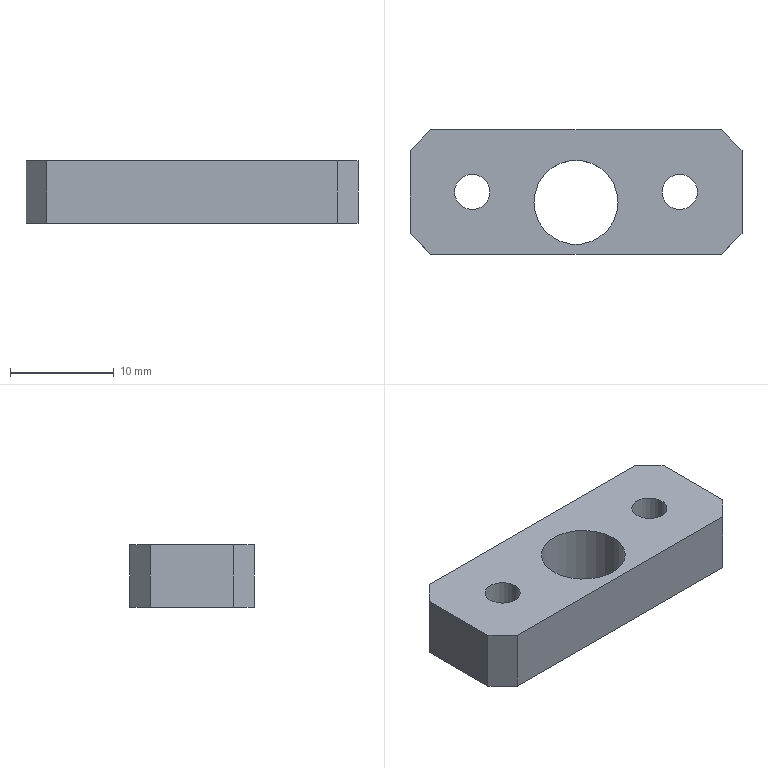Part | STEP file | 11-FG-SZ03211 | 1 solid | 22 faces | box 32 x 12 x 6 mm | volume 1674 mm3 | plane 12 | cylinder 10 | commonest cylinder face diameters 3.4 x4 6.5 x4 8.1 x2
STEP:
#1=CARTESIAN_POINT('',(4.05,-1.,6.));
#2=VERTEX_POINT('',#1);
#3=CARTESIAN_POINT('',(-4.05,-1.,6.));
#4=VERTEX_POINT('',#3);
#5=CARTESIAN_POINT('',(0.,-1.,6.));
#6=DIRECTION('',(0.,0.,-1.));
#7=DIRECTION('',(-1.,0.,0.));
#8=AXIS2_PLACEMENT_3D('',#5,#6,#7);
#9=CIRCLE('',#8,4.05);
#10=EDGE_CURVE('',#2,#4,#9,.T.);
#11=ORIENTED_EDGE('',*,*,#10,.F.);
#12=CARTESIAN_POINT('',(4.05,-1.,0.));
#13=VERTEX_POINT('',#12);
#14=CARTESIAN_POINT('',(4.05,-1.,6.));
#15=DIRECTION('',(0.,0.,-1.));
#16=VECTOR('',#15,1000.);
#17=LINE('',#14,#16);
#18=EDGE_CURVE('',#2,#13,#17,.T.);
#19=ORIENTED_EDGE('',*,*,#18,.T.);
#20=CARTESIAN_POINT('',(-4.05,-1.,0.));
#21=VERTEX_POINT('',#20);
#22=CARTESIAN_POINT('',(0.,-1.,0.));
#23=DIRECTION('',(0.,0.,-1.));
#24=DIRECTION('',(-1.,0.,0.));
#25=AXIS2_PLACEMENT_3D('',#22,#23,#24);
#26=CIRCLE('',#25,4.05);
#27=EDGE_CURVE('',#13,#21,#26,.T.);
#28=ORIENTED_EDGE('',*,*,#27,.T.);
#29=CARTESIAN_POINT('',(-4.05,-1.,6.));
#30=DIRECTION('',(0.,0.,-1.));
#31=VECTOR('',#30,1000.);
#32=LINE('',#29,#31);
#33=EDGE_CURVE('',#4,#21,#32,.T.);
#34=ORIENTED_EDGE('',*,*,#33,.F.);
#35=EDGE_LOOP('',(#11,#19,#28,#34));
#36=FACE_OUTER_BOUND('',#35,.T.);
#37=CARTESIAN_POINT('',(0.,-1.,6.));
#38=DIRECTION('',(0.,0.,-1.));
#39=DIRECTION('',(-1.,0.,0.));
#40=AXIS2_PLACEMENT_3D('',#37,#38,#39);
#41=CYLINDRICAL_SURFACE('',#40,4.05);
#42=ADVANCED_FACE('',(#36),#41,.F.);
#43=CARTESIAN_POINT('',(13.25,0.,3.4));
#44=VERTEX_POINT('',#43);
#45=CARTESIAN_POINT('',(6.75,0.,3.4));
#46=VERTEX_POINT('',#45);
#47=CARTESIAN_POINT('',(10.,0.,3.4));
#48=DIRECTION('',(0.,0.,-1.));
#49=DIRECTION('',(-1.,0.,0.));
#50=AXIS2_PLACEMENT_3D('',#47,#48,#49);
#51=CIRCLE('',#50,3.25);
#52=EDGE_CURVE('',#44,#46,#51,.T.);
#53=ORIENTED_EDGE('',*,*,#52,.F.);
#54=CARTESIAN_POINT('',(13.25,0.,0.));
#55=VERTEX_POINT('',#54);
#56=CARTESIAN_POINT('',(13.25,0.,0.));
#57=DIRECTION('',(0.,0.,-1.));
#58=VECTOR('',#57,1000.);
#59=LINE('',#56,#58);
#60=EDGE_CURVE('',#44,#55,#59,.T.);
#61=ORIENTED_EDGE('',*,*,#60,.T.);
#62=CARTESIAN_POINT('',(6.75,0.,0.));
#63=VERTEX_POINT('',#62);
#64=CARTESIAN_POINT('',(10.,0.,0.));
#65=DIRECTION('',(0.,0.,-1.));
#66=DIRECTION('',(-1.,0.,0.));
#67=AXIS2_PLACEMENT_3D('',#64,#65,#66);
#68=CIRCLE('',#67,3.25);
#69=EDGE_CURVE('',#55,#63,#68,.T.);
#70=ORIENTED_EDGE('',*,*,#69,.T.);
#71=CARTESIAN_POINT('',(6.75,0.,0.));
#72=DIRECTION('',(0.,0.,-1.));
#73=VECTOR('',#72,1000.);
#74=LINE('',#71,#73);
#75=EDGE_CURVE('',#46,#63,#74,.T.);
#76=ORIENTED_EDGE('',*,*,#75,.F.);
#77=EDGE_LOOP('',(#53,#61,#70,#76));
#78=FACE_OUTER_BOUND('',#77,.T.);
#79=CARTESIAN_POINT('',(10.,0.,0.));
#80=DIRECTION('',(0.,0.,-1.));
#81=DIRECTION('',(-1.,0.,0.));
#82=AXIS2_PLACEMENT_3D('',#79,#80,#81);
#83=CYLINDRICAL_SURFACE('',#82,3.25);
#84=ADVANCED_FACE('',(#78),#83,.F.);
#85=CARTESIAN_POINT('',(11.7,0.,6.));
#86=VERTEX_POINT('',#85);
#87=CARTESIAN_POINT('',(8.3,0.,6.));
#88=VERTEX_POINT('',#87);
#89=CARTESIAN_POINT('',(10.,0.,6.));
#90=DIRECTION('',(0.,0.,-1.));
#91=DIRECTION('',(-1.,0.,0.));
#92=AXIS2_PLACEMENT_3D('',#89,#90,#91);
#93=CIRCLE('',#92,1.7);
#94=EDGE_CURVE('',#86,#88,#93,.T.);
#95=ORIENTED_EDGE('',*,*,#94,.F.);
#96=CARTESIAN_POINT('',(11.7,0.,3.4));
#97=VERTEX_POINT('',#96);
#98=CARTESIAN_POINT('',(11.7,0.,0.));
#99=DIRECTION('',(0.,0.,-1.));
#100=VECTOR('',#99,1000.);
#101=LINE('',#98,#100);
#102=EDGE_CURVE('',#86,#97,#101,.T.);
#103=ORIENTED_EDGE('',*,*,#102,.T.);
#104=CARTESIAN_POINT('',(8.3,0.,3.4));
#105=VERTEX_POINT('',#104);
#106=CARTESIAN_POINT('',(10.,0.,3.4));
#107=DIRECTION('',(0.,0.,-1.));
#108=DIRECTION('',(-1.,0.,0.));
#109=AXIS2_PLACEMENT_3D('',#106,#107,#108);
#110=CIRCLE('',#109,1.7);
#111=EDGE_CURVE('',#97,#105,#110,.T.);
#112=ORIENTED_EDGE('',*,*,#111,.T.);
#113=CARTESIAN_POINT('',(8.3,0.,0.));
#114=DIRECTION('',(0.,0.,-1.));
#115=VECTOR('',#114,1000.);
#116=LINE('',#113,#115);
#117=EDGE_CURVE('',#88,#105,#116,.T.);
#118=ORIENTED_EDGE('',*,*,#117,.F.);
#119=EDGE_LOOP('',(#95,#103,#112,#118));
#120=FACE_OUTER_BOUND('',#119,.T.);
#121=CARTESIAN_POINT('',(10.,0.,0.));
#122=DIRECTION('',(0.,0.,-1.));
#123=DIRECTION('',(-1.,0.,0.));
#124=AXIS2_PLACEMENT_3D('',#121,#122,#123);
#125=CYLINDRICAL_SURFACE('',#124,1.7);
#126=ADVANCED_FACE('',(#120),#125,.F.);
#127=CARTESIAN_POINT('',(-6.75,0.,3.4));
#128=VERTEX_POINT('',#127);
#129=CARTESIAN_POINT('',(-13.25,0.,3.4));
#130=VERTEX_POINT('',#129);
#131=CARTESIAN_POINT('',(-10.,0.,3.4));
#132=DIRECTION('',(0.,0.,-1.));
#133=DIRECTION('',(-1.,0.,0.));
#134=AXIS2_PLACEMENT_3D('',#131,#132,#133);
#135=CIRCLE('',#134,3.25);
#136=EDGE_CURVE('',#128,#130,#135,.T.);
#137=ORIENTED_EDGE('',*,*,#136,.F.);
#138=CARTESIAN_POINT('',(-6.75,0.,0.));
#139=VERTEX_POINT('',#138);
#140=CARTESIAN_POINT('',(-6.75,0.,0.));
#141=DIRECTION('',(0.,0.,-1.));
#142=VECTOR('',#141,1000.);
#143=LINE('',#140,#142);
#144=EDGE_CURVE('',#128,#139,#143,.T.);
#145=ORIENTED_EDGE('',*,*,#144,.T.);
#146=CARTESIAN_POINT('',(-13.25,0.,0.));
#147=VERTEX_POINT('',#146);
#148=CARTESIAN_POINT('',(-10.,0.,0.));
#149=DIRECTION('',(0.,0.,-1.));
#150=DIRECTION('',(-1.,0.,0.));
#151=AXIS2_PLACEMENT_3D('',#148,#149,#150);
#152=CIRCLE('',#151,3.25);
#153=EDGE_CURVE('',#139,#147,#152,.T.);
#154=ORIENTED_EDGE('',*,*,#153,.T.);
#155=CARTESIAN_POINT('',(-13.25,0.,0.));
#156=DIRECTION('',(0.,0.,-1.));
#157=VECTOR('',#156,1000.);
#158=LINE('',#155,#157);
#159=EDGE_CURVE('',#130,#147,#158,.T.);
#160=ORIENTED_EDGE('',*,*,#159,.F.);
#161=EDGE_LOOP('',(#137,#145,#154,#160));
#162=FACE_OUTER_BOUND('',#161,.T.);
#163=CARTESIAN_POINT('',(-10.,0.,0.));
#164=DIRECTION('',(0.,0.,-1.));
#165=DIRECTION('',(-1.,0.,0.));
#166=AXIS2_PLACEMENT_3D('',#163,#164,#165);
#167=CYLINDRICAL_SURFACE('',#166,3.25);
#168=ADVANCED_FACE('',(#162),#167,.F.);
#169=CARTESIAN_POINT('',(-8.3,0.,6.));
#170=VERTEX_POINT('',#169);
#171=CARTESIAN_POINT('',(-11.7,0.,6.));
#172=VERTEX_POINT('',#171);
#173=CARTESIAN_POINT('',(-10.,0.,6.));
#174=DIRECTION('',(0.,0.,-1.));
#175=DIRECTION('',(-1.,0.,0.));
#176=AXIS2_PLACEMENT_3D('',#173,#174,#175);
#177=CIRCLE('',#176,1.7);
#178=EDGE_CURVE('',#170,#172,#177,.T.);
#179=ORIENTED_EDGE('',*,*,#178,.F.);
#180=CARTESIAN_POINT('',(-8.3,0.,3.4));
#181=VERTEX_POINT('',#180);
#182=CARTESIAN_POINT('',(-8.3,0.,0.));
#183=DIRECTION('',(0.,0.,-1.));
#184=VECTOR('',#183,1000.);
#185=LINE('',#182,#184);
#186=EDGE_CURVE('',#170,#181,#185,.T.);
#187=ORIENTED_EDGE('',*,*,#186,.T.);
#188=CARTESIAN_POINT('',(-11.7,0.,3.4));
#189=VERTEX_POINT('',#188);
#190=CARTESIAN_POINT('',(-10.,0.,3.4));
#191=DIRECTION('',(0.,0.,-1.));
#192=DIRECTION('',(-1.,0.,0.));
#193=AXIS2_PLACEMENT_3D('',#190,#191,#192);
#194=CIRCLE('',#193,1.7);
#195=EDGE_CURVE('',#181,#189,#194,.T.);
#196=ORIENTED_EDGE('',*,*,#195,.T.);
#197=CARTESIAN_POINT('',(-11.7,0.,0.));
#198=DIRECTION('',(0.,0.,-1.));
#199=VECTOR('',#198,1000.);
#200=LINE('',#197,#199);
#201=EDGE_CURVE('',#172,#189,#200,.T.);
#202=ORIENTED_EDGE('',*,*,#201,.F.);
#203=EDGE_LOOP('',(#179,#187,#196,#202));
#204=FACE_OUTER_BOUND('',#203,.T.);
#205=CARTESIAN_POINT('',(-10.,0.,0.));
#206=DIRECTION('',(0.,0.,-1.));
#207=DIRECTION('',(-1.,0.,0.));
#208=AXIS2_PLACEMENT_3D('',#205,#206,#207);
#209=CYLINDRICAL_SURFACE('',#208,1.7);
#210=ADVANCED_FACE('',(#204),#209,.F.);
#211=CARTESIAN_POINT('',(16.,-4.,6.));
#212=VERTEX_POINT('',#211);
#213=CARTESIAN_POINT('',(16.,4.,6.));
#214=VERTEX_POINT('',#213);
#215=CARTESIAN_POINT('',(16.,6.,6.));
#216=DIRECTION('',(0.,1.,0.));
#217=VECTOR('',#216,1000.);
#218=LINE('',#215,#217);
#219=EDGE_CURVE('',#212,#214,#218,.T.);
#220=ORIENTED_EDGE('',*,*,#219,.F.);
#221=CARTESIAN_POINT('',(16.,-4.,0.));
#222=VERTEX_POINT('',#221);
#223=CARTESIAN_POINT('',(16.,-4.,6.));
#224=DIRECTION('',(0.,0.,-1.));
#225=VECTOR('',#224,1000.);
#226=LINE('',#223,#225);
#227=EDGE_CURVE('',#212,#222,#226,.T.);
#228=ORIENTED_EDGE('',*,*,#227,.T.);
#229=CARTESIAN_POINT('',(16.,4.,0.));
#230=VERTEX_POINT('',#229);
#231=CARTESIAN_POINT('',(16.,6.,0.));
#232=DIRECTION('',(0.,1.,0.));
#233=VECTOR('',#232,1000.);
#234=LINE('',#231,#233);
#235=EDGE_CURVE('',#222,#230,#234,.T.);
#236=ORIENTED_EDGE('',*,*,#235,.T.);
#237=CARTESIAN_POINT('',(16.,4.,6.));
#238=DIRECTION('',(0.,0.,1.));
#239=VECTOR('',#238,1000.);
#240=LINE('',#237,#239);
#241=EDGE_CURVE('',#230,#214,#240,.T.);
#242=ORIENTED_EDGE('',*,*,#241,.T.);
#243=EDGE_LOOP('',(#220,#228,#236,#242));
#244=FACE_OUTER_BOUND('',#243,.T.);
#245=CARTESIAN_POINT('',(16.,6.,6.));
#246=DIRECTION('',(-1.,0.,0.));
#247=DIRECTION('',(0.,0.,1.));
#248=AXIS2_PLACEMENT_3D('',#245,#246,#247);
#249=PLANE('',#248);
#250=ADVANCED_FACE('',(#244),#249,.F.);
#251=CARTESIAN_POINT('',(14.,6.,0.));
#252=VERTEX_POINT('',#251);
#253=CARTESIAN_POINT('',(-14.,6.,0.));
#254=VERTEX_POINT('',#253);
#255=CARTESIAN_POINT('',(-16.,6.,0.));
#256=DIRECTION('',(-1.,0.,0.));
#257=VECTOR('',#256,1000.);
#258=LINE('',#255,#257);
#259=EDGE_CURVE('',#252,#254,#258,.T.);
#260=ORIENTED_EDGE('',*,*,#259,.T.);
#261=CARTESIAN_POINT('',(-14.,6.,6.));
#262=VERTEX_POINT('',#261);
#263=CARTESIAN_POINT('',(-14.,6.,6.));
#264=DIRECTION('',(0.,0.,1.));
#265=VECTOR('',#264,1000.);
#266=LINE('',#263,#265);
#267=EDGE_CURVE('',#254,#262,#266,.T.);
#268=ORIENTED_EDGE('',*,*,#267,.T.);
#269=CARTESIAN_POINT('',(14.,6.,6.));
#270=VERTEX_POINT('',#269);
#271=CARTESIAN_POINT('',(-16.,6.,6.));
#272=DIRECTION('',(-1.,0.,0.));
#273=VECTOR('',#272,1000.);
#274=LINE('',#271,#273);
#275=EDGE_CURVE('',#270,#262,#274,.T.);
#276=ORIENTED_EDGE('',*,*,#275,.F.);
#277=CARTESIAN_POINT('',(14.,6.,6.));
#278=DIRECTION('',(0.,0.,-1.));
#279=VECTOR('',#278,1000.);
#280=LINE('',#277,#279);
#281=EDGE_CURVE('',#270,#252,#280,.T.);
#282=ORIENTED_EDGE('',*,*,#281,.T.);
#283=EDGE_LOOP('',(#260,#268,#276,#282));
#284=FACE_OUTER_BOUND('',#283,.T.);
#285=CARTESIAN_POINT('',(-16.,6.,6.));
#286=DIRECTION('',(0.,-1.,0.));
#287=DIRECTION('',(0.,0.,-1.));
#288=AXIS2_PLACEMENT_3D('',#285,#286,#287);
#289=PLANE('',#288);
#290=ADVANCED_FACE('',(#284),#289,.F.);
#291=CARTESIAN_POINT('',(-16.,4.,0.));
#292=VERTEX_POINT('',#291);
#293=CARTESIAN_POINT('',(-16.,-4.,0.));
#294=VERTEX_POINT('',#293);
#295=CARTESIAN_POINT('',(-16.,6.,0.));
#296=DIRECTION('',(0.,-1.,0.));
#297=VECTOR('',#296,1000.);
#298=LINE('',#295,#297);
#299=EDGE_CURVE('',#292,#294,#298,.T.);
#300=ORIENTED_EDGE('',*,*,#299,.T.);
#301=CARTESIAN_POINT('',(-16.,-4.,6.));
#302=VERTEX_POINT('',#301);
#303=CARTESIAN_POINT('',(-16.,-4.,6.));
#304=DIRECTION('',(0.,0.,1.));
#305=VECTOR('',#304,1000.);
#306=LINE('',#303,#305);
#307=EDGE_CURVE('',#294,#302,#306,.T.);
#308=ORIENTED_EDGE('',*,*,#307,.T.);
#309=CARTESIAN_POINT('',(-16.,4.,6.));
#310=VERTEX_POINT('',#309);
#311=CARTESIAN_POINT('',(-16.,6.,6.));
#312=DIRECTION('',(0.,-1.,0.));
#313=VECTOR('',#312,1000.);
#314=LINE('',#311,#313);
#315=EDGE_CURVE('',#310,#302,#314,.T.);
#316=ORIENTED_EDGE('',*,*,#315,.F.);
#317=CARTESIAN_POINT('',(-16.,4.,6.));
#318=DIRECTION('',(0.,0.,-1.));
#319=VECTOR('',#318,1000.);
#320=LINE('',#317,#319);
#321=EDGE_CURVE('',#310,#292,#320,.T.);
#322=ORIENTED_EDGE('',*,*,#321,.T.);
#323=EDGE_LOOP('',(#300,#308,#316,#322));
#324=FACE_OUTER_BOUND('',#323,.T.);
#325=CARTESIAN_POINT('',(-16.,6.,6.));
#326=DIRECTION('',(1.,0.,0.));
#327=DIRECTION('',(0.,1.,0.));
#328=AXIS2_PLACEMENT_3D('',#325,#326,#327);
#329=PLANE('',#328);
#330=ADVANCED_FACE('',(#324),#329,.F.);
#331=CARTESIAN_POINT('',(-14.,-6.,6.));
#332=VERTEX_POINT('',#331);
#333=CARTESIAN_POINT('',(14.,-6.,6.));
#334=VERTEX_POINT('',#333);
#335=CARTESIAN_POINT('',(-16.,-6.,6.));
#336=DIRECTION('',(1.,0.,0.));
#337=VECTOR('',#336,1000.);
#338=LINE('',#335,#337);
#339=EDGE_CURVE('',#332,#334,#338,.T.);
#340=ORIENTED_EDGE('',*,*,#339,.F.);
#341=CARTESIAN_POINT('',(-14.,-6.,0.));
#342=VERTEX_POINT('',#341);
#343=CARTESIAN_POINT('',(-14.,-6.,6.));
#344=DIRECTION('',(0.,0.,-1.));
#345=VECTOR('',#344,1000.);
#346=LINE('',#343,#345);
#347=EDGE_CURVE('',#332,#342,#346,.T.);
#348=ORIENTED_EDGE('',*,*,#347,.T.);
#349=CARTESIAN_POINT('',(14.,-6.,0.));
#350=VERTEX_POINT('',#349);
#351=CARTESIAN_POINT('',(-16.,-6.,0.));
#352=DIRECTION('',(1.,0.,0.));
#353=VECTOR('',#352,1000.);
#354=LINE('',#351,#353);
#355=EDGE_CURVE('',#342,#350,#354,.T.);
#356=ORIENTED_EDGE('',*,*,#355,.T.);
#357=CARTESIAN_POINT('',(14.,-6.,6.));
#358=DIRECTION('',(0.,0.,1.));
#359=VECTOR('',#358,1000.);
#360=LINE('',#357,#359);
#361=EDGE_CURVE('',#350,#334,#360,.T.);
#362=ORIENTED_EDGE('',*,*,#361,.T.);
#363=EDGE_LOOP('',(#340,#348,#356,#362));
#364=FACE_OUTER_BOUND('',#363,.T.);
#365=CARTESIAN_POINT('',(-16.,-6.,6.));
#366=DIRECTION('',(0.,1.,0.));
#367=DIRECTION('',(0.,0.,1.));
#368=AXIS2_PLACEMENT_3D('',#365,#366,#367);
#369=PLANE('',#368);
#370=ADVANCED_FACE('',(#364),#369,.F.);
#371=CARTESIAN_POINT('',(0.,-1.,6.));
#372=DIRECTION('',(0.,0.,-1.));
#373=DIRECTION('',(-1.,0.,0.));
#374=AXIS2_PLACEMENT_3D('',#371,#372,#373);
#375=CIRCLE('',#374,4.05);
#376=EDGE_CURVE('',#4,#2,#375,.T.);
#377=ORIENTED_EDGE('',*,*,#376,.T.);
#378=ORIENTED_EDGE('',*,*,#10,.T.);
#379=EDGE_LOOP('',(#377,#378));
#380=FACE_BOUND('',#379,.T.);
#381=CARTESIAN_POINT('',(10.,0.,6.));
#382=DIRECTION('',(0.,0.,-1.));
#383=DIRECTION('',(-1.,0.,0.));
#384=AXIS2_PLACEMENT_3D('',#381,#382,#383);
#385=CIRCLE('',#384,1.7);
#386=EDGE_CURVE('',#88,#86,#385,.T.);
#387=ORIENTED_EDGE('',*,*,#386,.T.);
#388=ORIENTED_EDGE('',*,*,#94,.T.);
#389=EDGE_LOOP('',(#387,#388));
#390=FACE_BOUND('',#389,.T.);
#391=CARTESIAN_POINT('',(-10.,0.,6.));
#392=DIRECTION('',(0.,0.,-1.));
#393=DIRECTION('',(-1.,0.,0.));
#394=AXIS2_PLACEMENT_3D('',#391,#392,#393);
#395=CIRCLE('',#394,1.7);
#396=EDGE_CURVE('',#172,#170,#395,.T.);
#397=ORIENTED_EDGE('',*,*,#396,.T.);
#398=ORIENTED_EDGE('',*,*,#178,.T.);
#399=EDGE_LOOP('',(#397,#398));
#400=FACE_BOUND('',#399,.T.);
#401=ORIENTED_EDGE('',*,*,#315,.T.);
#402=CARTESIAN_POINT('',(-10.,-10.,6.));
#403=DIRECTION('',(0.7071,-0.7071,0.));
#404=VECTOR('',#403,1000.);
#405=LINE('',#402,#404);
#406=EDGE_CURVE('',#302,#332,#405,.T.);
#407=ORIENTED_EDGE('',*,*,#406,.T.);
#408=ORIENTED_EDGE('',*,*,#339,.T.);
#409=CARTESIAN_POINT('',(10.,-10.,6.));
#410=DIRECTION('',(0.7071,0.7071,0.));
#411=VECTOR('',#410,1000.);
#412=LINE('',#409,#411);
#413=EDGE_CURVE('',#334,#212,#412,.T.);
#414=ORIENTED_EDGE('',*,*,#413,.T.);
#415=ORIENTED_EDGE('',*,*,#219,.T.);
#416=CARTESIAN_POINT('',(10.,10.,6.));
#417=DIRECTION('',(-0.7071,0.7071,0.));
#418=VECTOR('',#417,1000.);
#419=LINE('',#416,#418);
#420=EDGE_CURVE('',#214,#270,#419,.T.);
#421=ORIENTED_EDGE('',*,*,#420,.T.);
#422=ORIENTED_EDGE('',*,*,#275,.T.);
#423=CARTESIAN_POINT('',(-10.,10.,6.));
#424=DIRECTION('',(-0.7071,-0.7071,0.));
#425=VECTOR('',#424,1000.);
#426=LINE('',#423,#425);
#427=EDGE_CURVE('',#262,#310,#426,.T.);
#428=ORIENTED_EDGE('',*,*,#427,.T.);
#429=EDGE_LOOP('',(#401,#407,#408,#414,#415,#421,#422,#428));
#430=FACE_OUTER_BOUND('',#429,.T.);
#431=CARTESIAN_POINT('',(0.,0.,6.));
#432=DIRECTION('',(0.,0.,1.));
#433=DIRECTION('',(1.,0.,0.));
#434=AXIS2_PLACEMENT_3D('',#431,#432,#433);
#435=PLANE('',#434);
#436=ADVANCED_FACE('',(#380,#390,#400,#430),#435,.T.);
#437=CARTESIAN_POINT('',(0.,-1.,0.));
#438=DIRECTION('',(0.,0.,-1.));
#439=DIRECTION('',(-1.,0.,0.));
#440=AXIS2_PLACEMENT_3D('',#437,#438,#439);
#441=CIRCLE('',#440,4.05);
#442=EDGE_CURVE('',#21,#13,#441,.T.);
#443=ORIENTED_EDGE('',*,*,#442,.F.);
#444=ORIENTED_EDGE('',*,*,#27,.F.);
#445=EDGE_LOOP('',(#443,#444));
#446=FACE_BOUND('',#445,.T.);
#447=CARTESIAN_POINT('',(10.,0.,0.));
#448=DIRECTION('',(0.,0.,-1.));
#449=DIRECTION('',(-1.,0.,0.));
#450=AXIS2_PLACEMENT_3D('',#447,#448,#449);
#451=CIRCLE('',#450,3.25);
#452=EDGE_CURVE('',#63,#55,#451,.T.);
#453=ORIENTED_EDGE('',*,*,#452,.F.);
#454=ORIENTED_EDGE('',*,*,#69,.F.);
#455=EDGE_LOOP('',(#453,#454));
#456=FACE_BOUND('',#455,.T.);
#457=CARTESIAN_POINT('',(-10.,0.,0.));
#458=DIRECTION('',(0.,0.,-1.));
#459=DIRECTION('',(-1.,0.,0.));
#460=AXIS2_PLACEMENT_3D('',#457,#458,#459);
#461=CIRCLE('',#460,3.25);
#462=EDGE_CURVE('',#147,#139,#461,.T.);
#463=ORIENTED_EDGE('',*,*,#462,.F.);
#464=ORIENTED_EDGE('',*,*,#153,.F.);
#465=EDGE_LOOP('',(#463,#464));
#466=FACE_BOUND('',#465,.T.);
#467=ORIENTED_EDGE('',*,*,#355,.F.);
#468=CARTESIAN_POINT('',(-14.,-6.,0.));
#469=DIRECTION('',(-0.7071,0.7071,0.));
#470=VECTOR('',#469,1000.);
#471=LINE('',#468,#470);
#472=EDGE_CURVE('',#342,#294,#471,.T.);
#473=ORIENTED_EDGE('',*,*,#472,.T.);
#474=ORIENTED_EDGE('',*,*,#299,.F.);
#475=CARTESIAN_POINT('',(-16.,4.,0.));
#476=DIRECTION('',(0.7071,0.7071,0.));
#477=VECTOR('',#476,1000.);
#478=LINE('',#475,#477);
#479=EDGE_CURVE('',#292,#254,#478,.T.);
#480=ORIENTED_EDGE('',*,*,#479,.T.);
#481=ORIENTED_EDGE('',*,*,#259,.F.);
#482=CARTESIAN_POINT('',(14.,6.,0.));
#483=DIRECTION('',(0.7071,-0.7071,0.));
#484=VECTOR('',#483,1000.);
#485=LINE('',#482,#484);
#486=EDGE_CURVE('',#252,#230,#485,.T.);
#487=ORIENTED_EDGE('',*,*,#486,.T.);
#488=ORIENTED_EDGE('',*,*,#235,.F.);
#489=CARTESIAN_POINT('',(16.,-4.,0.));
#490=DIRECTION('',(-0.7071,-0.7071,0.));
#491=VECTOR('',#490,1000.);
#492=LINE('',#489,#491);
#493=EDGE_CURVE('',#222,#350,#492,.T.);
#494=ORIENTED_EDGE('',*,*,#493,.T.);
#495=EDGE_LOOP('',(#467,#473,#474,#480,#481,#487,#488,#494));
#496=FACE_OUTER_BOUND('',#495,.T.);
#497=CARTESIAN_POINT('',(0.,0.,0.));
#498=DIRECTION('',(0.,0.,1.));
#499=DIRECTION('',(1.,0.,0.));
#500=AXIS2_PLACEMENT_3D('',#497,#498,#499);
#501=PLANE('',#500);
#502=ADVANCED_FACE('',(#446,#456,#466,#496),#501,.F.);
#503=ORIENTED_EDGE('',*,*,#186,.F.);
#504=ORIENTED_EDGE('',*,*,#396,.F.);
#505=ORIENTED_EDGE('',*,*,#201,.T.);
#506=CARTESIAN_POINT('',(-10.,0.,3.4));
#507=DIRECTION('',(0.,0.,-1.));
#508=DIRECTION('',(-1.,0.,0.));
#509=AXIS2_PLACEMENT_3D('',#506,#507,#508);
#510=CIRCLE('',#509,1.7);
#511=EDGE_CURVE('',#189,#181,#510,.T.);
#512=ORIENTED_EDGE('',*,*,#511,.T.);
#513=EDGE_LOOP('',(#503,#504,#505,#512));
#514=FACE_OUTER_BOUND('',#513,.T.);
#515=CARTESIAN_POINT('',(-10.,0.,0.));
#516=DIRECTION('',(0.,0.,-1.));
#517=DIRECTION('',(-1.,0.,0.));
#518=AXIS2_PLACEMENT_3D('',#515,#516,#517);
#519=CYLINDRICAL_SURFACE('',#518,1.7);
#520=ADVANCED_FACE('',(#514),#519,.F.);
#521=ORIENTED_EDGE('',*,*,#511,.F.);
#522=ORIENTED_EDGE('',*,*,#195,.F.);
#523=EDGE_LOOP('',(#521,#522));
#524=FACE_BOUND('',#523,.T.);
#525=CARTESIAN_POINT('',(-10.,0.,3.4));
#526=DIRECTION('',(0.,0.,-1.));
#527=DIRECTION('',(-1.,0.,0.));
#528=AXIS2_PLACEMENT_3D('',#525,#526,#527);
#529=CIRCLE('',#528,3.25);
#530=EDGE_CURVE('',#130,#128,#529,.T.);
#531=ORIENTED_EDGE('',*,*,#530,.T.);
#532=ORIENTED_EDGE('',*,*,#136,.T.);
#533=EDGE_LOOP('',(#531,#532));
#534=FACE_OUTER_BOUND('',#533,.T.);
#535=CARTESIAN_POINT('',(-8.3,0.,3.4));
#536=DIRECTION('',(0.,0.,1.));
#537=DIRECTION('',(1.,0.,0.));
#538=AXIS2_PLACEMENT_3D('',#535,#536,#537);
#539=PLANE('',#538);
#540=ADVANCED_FACE('',(#524,#534),#539,.F.);
#541=ORIENTED_EDGE('',*,*,#144,.F.);
#542=ORIENTED_EDGE('',*,*,#530,.F.);
#543=ORIENTED_EDGE('',*,*,#159,.T.);
#544=ORIENTED_EDGE('',*,*,#462,.T.);
#545=EDGE_LOOP('',(#541,#542,#543,#544));
#546=FACE_OUTER_BOUND('',#545,.T.);
#547=CARTESIAN_POINT('',(-10.,0.,0.));
#548=DIRECTION('',(0.,0.,-1.));
#549=DIRECTION('',(-1.,0.,0.));
#550=AXIS2_PLACEMENT_3D('',#547,#548,#549);
#551=CYLINDRICAL_SURFACE('',#550,3.25);
#552=ADVANCED_FACE('',(#546),#551,.F.);
#553=ORIENTED_EDGE('',*,*,#102,.F.);
#554=ORIENTED_EDGE('',*,*,#386,.F.);
#555=ORIENTED_EDGE('',*,*,#117,.T.);
#556=CARTESIAN_POINT('',(10.,0.,3.4));
#557=DIRECTION('',(0.,0.,-1.));
#558=DIRECTION('',(-1.,0.,0.));
#559=AXIS2_PLACEMENT_3D('',#556,#557,#558);
#560=CIRCLE('',#559,1.7);
#561=EDGE_CURVE('',#105,#97,#560,.T.);
#562=ORIENTED_EDGE('',*,*,#561,.T.);
#563=EDGE_LOOP('',(#553,#554,#555,#562));
#564=FACE_OUTER_BOUND('',#563,.T.);
#565=CARTESIAN_POINT('',(10.,0.,0.));
#566=DIRECTION('',(0.,0.,-1.));
#567=DIRECTION('',(-1.,0.,0.));
#568=AXIS2_PLACEMENT_3D('',#565,#566,#567);
#569=CYLINDRICAL_SURFACE('',#568,1.7);
#570=ADVANCED_FACE('',(#564),#569,.F.);
#571=ORIENTED_EDGE('',*,*,#561,.F.);
#572=ORIENTED_EDGE('',*,*,#111,.F.);
#573=EDGE_LOOP('',(#571,#572));
#574=FACE_BOUND('',#573,.T.);
#575=CARTESIAN_POINT('',(10.,0.,3.4));
#576=DIRECTION('',(0.,0.,-1.));
#577=DIRECTION('',(-1.,0.,0.));
#578=AXIS2_PLACEMENT_3D('',#575,#576,#577);
#579=CIRCLE('',#578,3.25);
#580=EDGE_CURVE('',#46,#44,#579,.T.);
#581=ORIENTED_EDGE('',*,*,#580,.T.);
#582=ORIENTED_EDGE('',*,*,#52,.T.);
#583=EDGE_LOOP('',(#581,#582));
#584=FACE_OUTER_BOUND('',#583,.T.);
#585=CARTESIAN_POINT('',(11.7,0.,3.4));
#586=DIRECTION('',(0.,0.,1.));
#587=DIRECTION('',(1.,0.,0.));
#588=AXIS2_PLACEMENT_3D('',#585,#586,#587);
#589=PLANE('',#588);
#590=ADVANCED_FACE('',(#574,#584),#589,.F.);
#591=ORIENTED_EDGE('',*,*,#60,.F.);
#592=ORIENTED_EDGE('',*,*,#580,.F.);
#593=ORIENTED_EDGE('',*,*,#75,.T.);
#594=ORIENTED_EDGE('',*,*,#452,.T.);
#595=EDGE_LOOP('',(#591,#592,#593,#594));
#596=FACE_OUTER_BOUND('',#595,.T.);
#597=CARTESIAN_POINT('',(10.,0.,0.));
#598=DIRECTION('',(0.,0.,-1.));
#599=DIRECTION('',(-1.,0.,0.));
#600=AXIS2_PLACEMENT_3D('',#597,#598,#599);
#601=CYLINDRICAL_SURFACE('',#600,3.25);
#602=ADVANCED_FACE('',(#596),#601,.F.);
#603=ORIENTED_EDGE('',*,*,#18,.F.);
#604=ORIENTED_EDGE('',*,*,#376,.F.);
#605=ORIENTED_EDGE('',*,*,#33,.T.);
#606=ORIENTED_EDGE('',*,*,#442,.T.);
#607=EDGE_LOOP('',(#603,#604,#605,#606));
#608=FACE_OUTER_BOUND('',#607,.T.);
#609=CARTESIAN_POINT('',(0.,-1.,6.));
#610=DIRECTION('',(0.,0.,-1.));
#611=DIRECTION('',(-1.,0.,0.));
#612=AXIS2_PLACEMENT_3D('',#609,#610,#611);
#613=CYLINDRICAL_SURFACE('',#612,4.05);
#614=ADVANCED_FACE('',(#608),#613,.F.);
#615=ORIENTED_EDGE('',*,*,#406,.F.);
#616=ORIENTED_EDGE('',*,*,#307,.F.);
#617=ORIENTED_EDGE('',*,*,#472,.F.);
#618=ORIENTED_EDGE('',*,*,#347,.F.);
#619=EDGE_LOOP('',(#615,#616,#617,#618));
#620=FACE_OUTER_BOUND('',#619,.T.);
#621=CARTESIAN_POINT('',(-14.,-6.,6.));
#622=DIRECTION('',(0.7071,0.7071,0.));
#623=DIRECTION('',(0.,0.,-1.));
#624=AXIS2_PLACEMENT_3D('',#621,#622,#623);
#625=PLANE('',#624);
#626=ADVANCED_FACE('',(#620),#625,.F.);
#627=ORIENTED_EDGE('',*,*,#413,.F.);
#628=ORIENTED_EDGE('',*,*,#361,.F.);
#629=ORIENTED_EDGE('',*,*,#493,.F.);
#630=ORIENTED_EDGE('',*,*,#227,.F.);
#631=EDGE_LOOP('',(#627,#628,#629,#630));
#632=FACE_OUTER_BOUND('',#631,.T.);
#633=CARTESIAN_POINT('',(16.,-4.,6.));
#634=DIRECTION('',(-0.7071,0.7071,0.));
#635=DIRECTION('',(0.,0.,-1.));
#636=AXIS2_PLACEMENT_3D('',#633,#634,#635);
#637=PLANE('',#636);
#638=ADVANCED_FACE('',(#632),#637,.F.);
#639=ORIENTED_EDGE('',*,*,#427,.F.);
#640=ORIENTED_EDGE('',*,*,#267,.F.);
#641=ORIENTED_EDGE('',*,*,#479,.F.);
#642=ORIENTED_EDGE('',*,*,#321,.F.);
#643=EDGE_LOOP('',(#639,#640,#641,#642));
#644=FACE_OUTER_BOUND('',#643,.T.);
#645=CARTESIAN_POINT('',(-16.,4.,6.));
#646=DIRECTION('',(0.7071,-0.7071,0.));
#647=DIRECTION('',(0.,0.,-1.));
#648=AXIS2_PLACEMENT_3D('',#645,#646,#647);
#649=PLANE('',#648);
#650=ADVANCED_FACE('',(#644),#649,.F.);
#651=ORIENTED_EDGE('',*,*,#420,.F.);
#652=ORIENTED_EDGE('',*,*,#241,.F.);
#653=ORIENTED_EDGE('',*,*,#486,.F.);
#654=ORIENTED_EDGE('',*,*,#281,.F.);
#655=EDGE_LOOP('',(#651,#652,#653,#654));
#656=FACE_OUTER_BOUND('',#655,.T.);
#657=CARTESIAN_POINT('',(14.,6.,6.));
#658=DIRECTION('',(-0.7071,-0.7071,0.));
#659=DIRECTION('',(0.,0.,-1.));
#660=AXIS2_PLACEMENT_3D('',#657,#658,#659);
#661=PLANE('',#660);
#662=ADVANCED_FACE('',(#656),#661,.F.);
#663=CLOSED_SHELL('',(#42,#84,#126,#168,#210,#250,#290,#330,#370,#436,#502,#520,#540,#552,#570,#590,#602,#614,#626,#638,#650,#662));
#664=MANIFOLD_SOLID_BREP('',#663);
#665=CARTESIAN_POINT('',(0.,0.,0.));
#666=DIRECTION('',(0.,0.,1.));
#667=DIRECTION('',(1.,0.,0.));
#668=AXIS2_PLACEMENT_3D('',#665,#666,#667);
#669=(LENGTH_UNIT()NAMED_UNIT(*)SI_UNIT(.MILLI.,.METRE.));
#670=UNCERTAINTY_MEASURE_WITH_UNIT(LENGTH_MEASURE(0.00001),#669,'','');
#671=(NAMED_UNIT(*)PLANE_ANGLE_UNIT()SI_UNIT($,.RADIAN.));
#672=(NAMED_UNIT(*)SI_UNIT($,.STERADIAN.)SOLID_ANGLE_UNIT());
#673=(GEOMETRIC_REPRESENTATION_CONTEXT(3)GLOBAL_UNCERTAINTY_ASSIGNED_CONTEXT((#670))GLOBAL_UNIT_ASSIGNED_CONTEXT((#669,#671,#672))REPRESENTATION_CONTEXT('',''));
#674=ADVANCED_BREP_SHAPE_REPRESENTATION('',(#664,#668),#673);